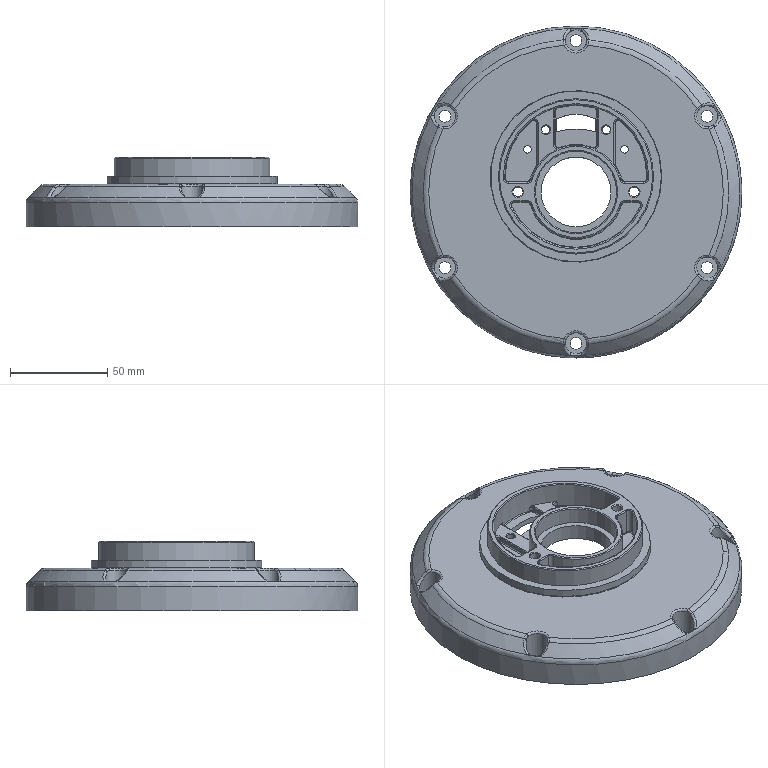NC program | NX | posted with a generic post | part box 171 x 171 x 36 mm
Whole program:
N10 G17 G21 G94 G90
(底壁铣开粗_COPY_1_COPY_COPY_1 , TOOL : D4J-L24)
N12 T09 M6
N14 G54
N16 G17 G0 G90 X22.4 Y25.068 S4000 M3
N18 G43 Z20. H9
N20 Z-13.5
N22 G94 G1 Z-14. F600.
N24 G3 X21.9 Y24.568 R0.5
N26 G1 Y14.043
N28 X21.894 Y14.012
N30 X21.916 Y13.99
N32 G2 X25.02 Y7.073 R26.
N34 G1 X25.032 Y7.028
N36 X25.07 Y7.
N38 X25.116
N40 X34.889
N42 X34.943 Y7.004
N44 X34.983 Y7.043
N46 X34.988 Y7.097
N48 G3 X34.998 Y7.674 R35.
N50 X22.063 Y35.17 R35.
N52 X21.9 Y35.093 R0.1
N54 G1 Y24.568
N56 Y23.568
N58 G3 X22.4 Y23.068 R0.5
N60 G1 Z-13.5
N62 G0 Z20.
N64 X8.6 Y32.609
N66 Z-13.5
N68 G1 Z-14.
N70 G3 X9.1 Y33.109 R0.5
N72 G1 Y41.72
N74 Y41.766
N76 X9.071 Y41.804
N78 X9.026 Y41.816
N80 G3 X-9.026 Y41.816 R35.
N82 G1 X-9.071 Y41.804
N84 X-9.1 Y41.766
N86 Y41.72
N88 Y24.499
N90 X-9.088 Y24.433
N92 X-9.031 Y24.394
N94 X-8.966 Y24.405
N96 G2 X8.966 Y24.405 R26.
N98 G1 X9.031 Y24.394
N100 X9.088 Y24.433
N102 X9.1 Y24.499
N104 Y33.109
N106 Y34.109
N108 G3 X8.6 Y34.609 R0.5
N110 G1 Z-13.5
N112 G0 Z20.
N114 X-22.4 Y24.068
N116 Z-13.5
N118 G1 Z-14.
N120 G3 X-21.9 Y24.568 R0.5
N122 G1 Y35.093
N124 G3 X-22.063 Y35.17 R0.1
N126 X-34.988 Y7.097 R35.
N128 G1 X-34.983 Y7.043
N130 X-34.943 Y7.004
N132 X-34.889 Y7.
N134 X-25.116
N136 X-25.07
N138 X-25.032 Y7.028
N140 X-25.02 Y7.073
N142 G2 X-21.916 Y13.99 R26.
N144 G1 X-21.894 Y14.012
N146 X-21.9 Y14.043
N148 Y24.568
N150 Y25.568
N152 G3 X-22.4 Y26.068 R0.5
N154 G1 Z-13.5
N156 G0 Z20.
N158 X-27.79 Y-7.5
N160 Z-13.5
N162 G1 Z-14.
N164 G3 X-28.29 Y-7. R0.5
N166 G1 X-31.465
N168 G3 X-31.555 Y-7.143 R0.1
N170 X31.555 Y-7.143 R35.
N172 X31.465 Y-7. R0.1
N174 G1 X25.115
N176 X25.07
N178 X25.032 Y-7.028
N180 X25.02 Y-7.073
N182 G2 X-25.02 Y-7.073 R26.
N184 G1 X-25.032 Y-7.028
N186 X-25.07 Y-7.
N188 X-25.115
N190 X-28.29
N192 X-29.29
N194 G3 X-29.79 Y-7.5 R0.5
N196 G1 Z-13.5
N198 G0 Z20.
N200 M5
(底壁铣开粗_COPY_COPY_2 , TOOL : D10R0.2-L30)
N202 T11 M6
N204 G54
N206 G17 G0 G90 X4.5 Y-53.457 S4000 M3
N208 G43 Z20. H11
N210 Z-13.45
N212 G94 G2 X4.5 Y-53.457 Z-13.672 I-4.5 J-0.043 F750.
N214 X4.5 Y-53.457 Z-13.894 I-4.5 J-0.043
N216 X0. Y-58. Z-13.95 R4.5
N218 X-57.304 Y-8.958 R58.
N220 X-57.028 Y-8.431 R0.5
N222 G1 X-56.16 Y-8.009
N224 G3 X-55.878 Y-7.55 R0.5
N226 G2 X-51.39 Y-6.321 R2.4
N228 G1 X-35.129 Y-35.04
N230 G2 X-36.034 Y-38.311 R2.4
N232 X-39.305 Y-37.405 R2.4
N234 G1 X-54.997 Y-9.693
N236 G3 X-55.411 Y-9.44 R0.5
N238 G1 X-56.831 Y-9.38
N240 G2 X-57.304 Y-8.958 R0.5
N242 X-20.473 Y54.267 R58.
N244 X-20.397 Y54.082 R0.1
N246 G3 X20.811 Y53.896 R-50.394
N248 X20.214 Y53.668 R0.45
N250 G1 X20.054 Y53.308
N252 G3 X20.305 Y52.65 R0.5
N254 G2 X19.623 Y52.954 R-49.05
N256 G3 X20.072 Y52.979 R0.5
N258 G1 X20.442 Y53.192
N260 G3 X20.397 Y54.082 R0.5
N262 G2 X20.473 Y54.267 R0.1
N264 X57.304 Y-8.958 R58.
N266 X56.831 Y-9.38 R0.5
N268 G1 X55.411 Y-9.44
N270 G3 X54.997 Y-9.693 R0.5
N272 G1 X39.305 Y-37.405
N274 G2 X36.034 Y-38.311 R2.4
N276 X35.129 Y-35.04 R2.4
N278 G1 X51.39 Y-6.321
N280 G2 X55.878 Y-7.55 R2.4
N282 G3 X56.16 Y-8.009 R0.5
N284 G1 X57.028 Y-8.431
N286 G2 X57.304 Y-8.958 R0.5
N288 X-4.994 Y-57.785 R58.
N290 X-5.439 Y-57.395 R0.5
N292 G1 X-6.825 Y-51.152
N294 G3 X-7.242 Y-50.766 R0.5
N296 G2 X-34.799 Y-37.665 R51.28
N298 X-34.606 Y-37.436 R0.15
N300 G3 X34.606 Y-37.436 R57.114
N302 G2 X34.799 Y-37.665 R0.15
N304 X-4.415 Y-51.09 R51.28
N306 X-5.411 Y-50.994 R51.28
N308 G1 Z-13.45
N310 G0 Z20.
(底壁铣开粗_COPY_COPY_COPY , TOOL : D10R0.2-L30)
N312 X-53.942 Y5.5
N314 Z-13.45
N316 G1 Z-13.95
N318 X-51.5
N320 G3 X-49. Y8. R2.5
N322 G2 X0. Y57. R49.
N324 X-49. Y8. R-49.
N326 X-48.99 Y9. R49.
N328 G3 X-51.438 Y11.55 R2.5
N330 G1 X-53.88 Y11.6
N332 Z-13.45
N334 G0 Z20.
N336 M5
N338 M2